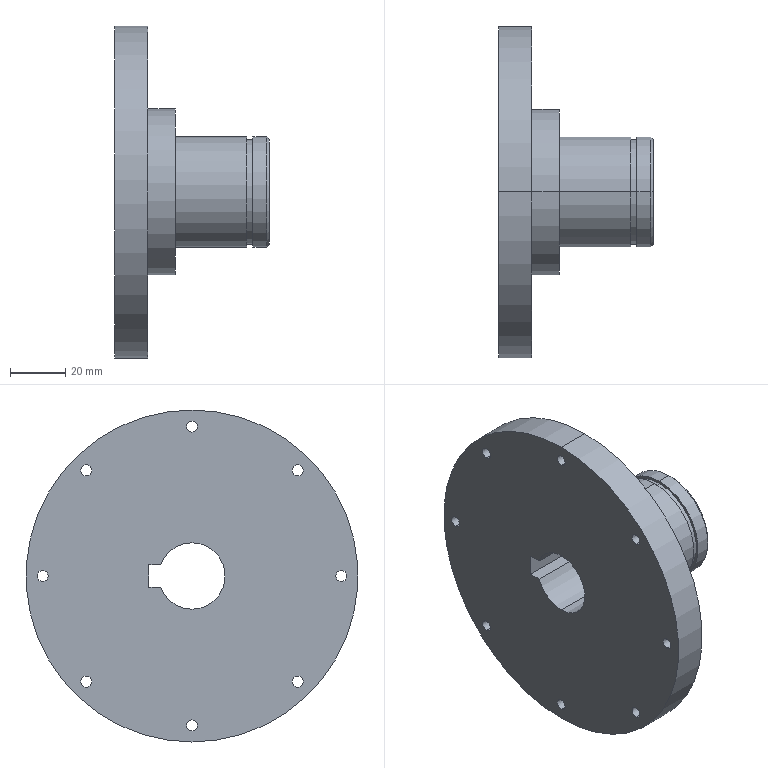Part | SolidWorks | features ICE 3, RevolutionThin 3, Chamfer 1 | 1 solid | 40 faces | box 56 x 120 x 120 mm | volume 178131 mm3 | cylinder 29 | plane 9 | cone 2 | commonest cylinder face diameters 4 x16 40 x4 24 x3 38 x2 60 x2 120 x2
STEP:
#1=CARTESIAN_POINT('',(56.,0.,-19.));
#2=VERTEX_POINT('',#1);
#3=CARTESIAN_POINT('',(56.,0.,19.));
#4=VERTEX_POINT('',#3);
#5=CARTESIAN_POINT('',(56.,0.,0.));
#6=DIRECTION('',(1.,0.,0.));
#7=DIRECTION('',(0.,0.,1.));
#8=AXIS2_PLACEMENT_3D('',#5,#6,#7);
#9=CIRCLE('',#8,19.);
#10=EDGE_CURVE('',#2,#4,#9,.T.);
#11=ORIENTED_EDGE('',*,*,#10,.F.);
#12=CARTESIAN_POINT('',(55.,0.,-20.));
#13=VERTEX_POINT('',#12);
#14=CARTESIAN_POINT('',(55.,0.,-20.));
#15=DIRECTION('',(-0.7071,0.,-0.7071));
#16=VECTOR('',#15,1000.);
#17=LINE('',#14,#16);
#18=EDGE_CURVE('',#2,#13,#17,.T.);
#19=ORIENTED_EDGE('',*,*,#18,.T.);
#20=CARTESIAN_POINT('',(55.,0.,20.));
#21=VERTEX_POINT('',#20);
#22=CARTESIAN_POINT('',(55.,0.,0.));
#23=DIRECTION('',(-1.,0.,0.));
#24=DIRECTION('',(0.,0.,1.));
#25=AXIS2_PLACEMENT_3D('',#22,#23,#24);
#26=CIRCLE('',#25,20.);
#27=EDGE_CURVE('',#21,#13,#26,.T.);
#28=ORIENTED_EDGE('',*,*,#27,.F.);
#29=CARTESIAN_POINT('',(55.,0.,20.));
#30=DIRECTION('',(-0.7071,0.,0.7071));
#31=VECTOR('',#30,1000.);
#32=LINE('',#29,#31);
#33=EDGE_CURVE('',#4,#21,#32,.T.);
#34=ORIENTED_EDGE('',*,*,#33,.F.);
#35=EDGE_LOOP('',(#11,#19,#28,#34));
#36=FACE_OUTER_BOUND('',#35,.T.);
#37=CARTESIAN_POINT('',(55.,0.,0.));
#38=DIRECTION('',(-1.,0.,0.));
#39=DIRECTION('',(0.,0.,1.));
#40=AXIS2_PLACEMENT_3D('',#37,#38,#39);
#41=CONICAL_SURFACE('',#40,20.,0.7854);
#42=ADVANCED_FACE('',(#36),#41,.T.);
#43=CARTESIAN_POINT('',(12.,54.,-2.));
#44=VERTEX_POINT('',#43);
#45=CARTESIAN_POINT('',(12.,54.,2.));
#46=VERTEX_POINT('',#45);
#47=CARTESIAN_POINT('',(12.,54.,0.));
#48=DIRECTION('',(-1.,0.,0.));
#49=DIRECTION('',(0.,0.,1.));
#50=AXIS2_PLACEMENT_3D('',#47,#48,#49);
#51=CIRCLE('',#50,2.);
#52=EDGE_CURVE('',#44,#46,#51,.T.);
#53=ORIENTED_EDGE('',*,*,#52,.F.);
#54=CARTESIAN_POINT('',(0.,54.,-2.));
#55=VERTEX_POINT('',#54);
#56=CARTESIAN_POINT('',(56.,54.,-2.));
#57=DIRECTION('',(-1.,0.,0.));
#58=VECTOR('',#57,1000.);
#59=LINE('',#56,#58);
#60=EDGE_CURVE('',#44,#55,#59,.T.);
#61=ORIENTED_EDGE('',*,*,#60,.T.);
#62=CARTESIAN_POINT('',(0.,54.,2.));
#63=VERTEX_POINT('',#62);
#64=CARTESIAN_POINT('',(0.,54.,0.));
#65=DIRECTION('',(-1.,0.,0.));
#66=DIRECTION('',(0.,0.,1.));
#67=AXIS2_PLACEMENT_3D('',#64,#65,#66);
#68=CIRCLE('',#67,2.);
#69=EDGE_CURVE('',#55,#63,#68,.T.);
#70=ORIENTED_EDGE('',*,*,#69,.T.);
#71=CARTESIAN_POINT('',(56.,54.,2.));
#72=DIRECTION('',(-1.,0.,0.));
#73=VECTOR('',#72,1000.);
#74=LINE('',#71,#73);
#75=EDGE_CURVE('',#46,#63,#74,.T.);
#76=ORIENTED_EDGE('',*,*,#75,.F.);
#77=EDGE_LOOP('',(#53,#61,#70,#76));
#78=FACE_OUTER_BOUND('',#77,.T.);
#79=CARTESIAN_POINT('',(56.,54.,0.));
#80=DIRECTION('',(-1.,0.,0.));
#81=DIRECTION('',(0.,0.,1.));
#82=AXIS2_PLACEMENT_3D('',#79,#80,#81);
#83=CYLINDRICAL_SURFACE('',#82,2.);
#84=ADVANCED_FACE('',(#78),#83,.F.);
#85=CARTESIAN_POINT('',(12.,38.184,36.184));
#86=VERTEX_POINT('',#85);
#87=CARTESIAN_POINT('',(12.,38.184,40.184));
#88=VERTEX_POINT('',#87);
#89=CARTESIAN_POINT('',(12.,38.184,38.184));
#90=DIRECTION('',(-1.,0.,0.));
#91=DIRECTION('',(0.,0.,1.));
#92=AXIS2_PLACEMENT_3D('',#89,#90,#91);
#93=CIRCLE('',#92,2.);
#94=EDGE_CURVE('',#86,#88,#93,.T.);
#95=ORIENTED_EDGE('',*,*,#94,.F.);
#96=CARTESIAN_POINT('',(0.,38.184,36.184));
#97=VERTEX_POINT('',#96);
#98=CARTESIAN_POINT('',(56.,38.184,36.184));
#99=DIRECTION('',(-1.,0.,0.));
#100=VECTOR('',#99,1000.);
#101=LINE('',#98,#100);
#102=EDGE_CURVE('',#86,#97,#101,.T.);
#103=ORIENTED_EDGE('',*,*,#102,.T.);
#104=CARTESIAN_POINT('',(0.,38.184,40.184));
#105=VERTEX_POINT('',#104);
#106=CARTESIAN_POINT('',(0.,38.184,38.184));
#107=DIRECTION('',(-1.,0.,0.));
#108=DIRECTION('',(0.,0.,1.));
#109=AXIS2_PLACEMENT_3D('',#106,#107,#108);
#110=CIRCLE('',#109,2.);
#111=EDGE_CURVE('',#97,#105,#110,.T.);
#112=ORIENTED_EDGE('',*,*,#111,.T.);
#113=CARTESIAN_POINT('',(56.,38.184,40.184));
#114=DIRECTION('',(-1.,0.,0.));
#115=VECTOR('',#114,1000.);
#116=LINE('',#113,#115);
#117=EDGE_CURVE('',#88,#105,#116,.T.);
#118=ORIENTED_EDGE('',*,*,#117,.F.);
#119=EDGE_LOOP('',(#95,#103,#112,#118));
#120=FACE_OUTER_BOUND('',#119,.T.);
#121=CARTESIAN_POINT('',(56.,38.184,38.184));
#122=DIRECTION('',(-1.,0.,0.));
#123=DIRECTION('',(0.,0.,1.));
#124=AXIS2_PLACEMENT_3D('',#121,#122,#123);
#125=CYLINDRICAL_SURFACE('',#124,2.);
#126=ADVANCED_FACE('',(#120),#125,.F.);
#127=CARTESIAN_POINT('',(12.,0.,52.));
#128=VERTEX_POINT('',#127);
#129=CARTESIAN_POINT('',(12.,0.,56.));
#130=VERTEX_POINT('',#129);
#131=CARTESIAN_POINT('',(12.,0.,54.));
#132=DIRECTION('',(-1.,0.,0.));
#133=DIRECTION('',(0.,0.,1.));
#134=AXIS2_PLACEMENT_3D('',#131,#132,#133);
#135=CIRCLE('',#134,2.);
#136=EDGE_CURVE('',#128,#130,#135,.T.);
#137=ORIENTED_EDGE('',*,*,#136,.F.);
#138=CARTESIAN_POINT('',(0.,0.,52.));
#139=VERTEX_POINT('',#138);
#140=CARTESIAN_POINT('',(56.,0.,52.));
#141=DIRECTION('',(-1.,0.,0.));
#142=VECTOR('',#141,1000.);
#143=LINE('',#140,#142);
#144=EDGE_CURVE('',#128,#139,#143,.T.);
#145=ORIENTED_EDGE('',*,*,#144,.T.);
#146=CARTESIAN_POINT('',(0.,0.,56.));
#147=VERTEX_POINT('',#146);
#148=CARTESIAN_POINT('',(0.,0.,54.));
#149=DIRECTION('',(-1.,0.,0.));
#150=DIRECTION('',(0.,0.,1.));
#151=AXIS2_PLACEMENT_3D('',#148,#149,#150);
#152=CIRCLE('',#151,2.);
#153=EDGE_CURVE('',#139,#147,#152,.T.);
#154=ORIENTED_EDGE('',*,*,#153,.T.);
#155=CARTESIAN_POINT('',(56.,0.,56.));
#156=DIRECTION('',(-1.,0.,0.));
#157=VECTOR('',#156,1000.);
#158=LINE('',#155,#157);
#159=EDGE_CURVE('',#130,#147,#158,.T.);
#160=ORIENTED_EDGE('',*,*,#159,.F.);
#161=EDGE_LOOP('',(#137,#145,#154,#160));
#162=FACE_OUTER_BOUND('',#161,.T.);
#163=CARTESIAN_POINT('',(56.,0.,54.));
#164=DIRECTION('',(-1.,0.,0.));
#165=DIRECTION('',(0.,0.,1.));
#166=AXIS2_PLACEMENT_3D('',#163,#164,#165);
#167=CYLINDRICAL_SURFACE('',#166,2.);
#168=ADVANCED_FACE('',(#162),#167,.F.);
#169=CARTESIAN_POINT('',(12.,-38.184,36.184));
#170=VERTEX_POINT('',#169);
#171=CARTESIAN_POINT('',(12.,-38.184,40.184));
#172=VERTEX_POINT('',#171);
#173=CARTESIAN_POINT('',(12.,-38.184,38.184));
#174=DIRECTION('',(-1.,0.,0.));
#175=DIRECTION('',(0.,0.,1.));
#176=AXIS2_PLACEMENT_3D('',#173,#174,#175);
#177=CIRCLE('',#176,2.);
#178=EDGE_CURVE('',#170,#172,#177,.T.);
#179=ORIENTED_EDGE('',*,*,#178,.F.);
#180=CARTESIAN_POINT('',(0.,-38.184,36.184));
#181=VERTEX_POINT('',#180);
#182=CARTESIAN_POINT('',(56.,-38.184,36.184));
#183=DIRECTION('',(-1.,0.,0.));
#184=VECTOR('',#183,1000.);
#185=LINE('',#182,#184);
#186=EDGE_CURVE('',#170,#181,#185,.T.);
#187=ORIENTED_EDGE('',*,*,#186,.T.);
#188=CARTESIAN_POINT('',(0.,-38.184,40.184));
#189=VERTEX_POINT('',#188);
#190=CARTESIAN_POINT('',(0.,-38.184,38.184));
#191=DIRECTION('',(-1.,0.,0.));
#192=DIRECTION('',(0.,0.,1.));
#193=AXIS2_PLACEMENT_3D('',#190,#191,#192);
#194=CIRCLE('',#193,2.);
#195=EDGE_CURVE('',#181,#189,#194,.T.);
#196=ORIENTED_EDGE('',*,*,#195,.T.);
#197=CARTESIAN_POINT('',(56.,-38.184,40.184));
#198=DIRECTION('',(-1.,0.,0.));
#199=VECTOR('',#198,1000.);
#200=LINE('',#197,#199);
#201=EDGE_CURVE('',#172,#189,#200,.T.);
#202=ORIENTED_EDGE('',*,*,#201,.F.);
#203=EDGE_LOOP('',(#179,#187,#196,#202));
#204=FACE_OUTER_BOUND('',#203,.T.);
#205=CARTESIAN_POINT('',(56.,-38.184,38.184));
#206=DIRECTION('',(-1.,0.,0.));
#207=DIRECTION('',(0.,0.,1.));
#208=AXIS2_PLACEMENT_3D('',#205,#206,#207);
#209=CYLINDRICAL_SURFACE('',#208,2.);
#210=ADVANCED_FACE('',(#204),#209,.F.);
#211=CARTESIAN_POINT('',(12.,-54.,-2.));
#212=VERTEX_POINT('',#211);
#213=CARTESIAN_POINT('',(12.,-54.,2.));
#214=VERTEX_POINT('',#213);
#215=CARTESIAN_POINT('',(12.,-54.,0.));
#216=DIRECTION('',(-1.,0.,0.));
#217=DIRECTION('',(0.,0.,1.));
#218=AXIS2_PLACEMENT_3D('',#215,#216,#217);
#219=CIRCLE('',#218,2.);
#220=EDGE_CURVE('',#212,#214,#219,.T.);
#221=ORIENTED_EDGE('',*,*,#220,.F.);
#222=CARTESIAN_POINT('',(0.,-54.,-2.));
#223=VERTEX_POINT('',#222);
#224=CARTESIAN_POINT('',(56.,-54.,-2.));
#225=DIRECTION('',(-1.,0.,0.));
#226=VECTOR('',#225,1000.);
#227=LINE('',#224,#226);
#228=EDGE_CURVE('',#212,#223,#227,.T.);
#229=ORIENTED_EDGE('',*,*,#228,.T.);
#230=CARTESIAN_POINT('',(0.,-54.,2.));
#231=VERTEX_POINT('',#230);
#232=CARTESIAN_POINT('',(0.,-54.,0.));
#233=DIRECTION('',(-1.,0.,0.));
#234=DIRECTION('',(0.,0.,1.));
#235=AXIS2_PLACEMENT_3D('',#232,#233,#234);
#236=CIRCLE('',#235,2.);
#237=EDGE_CURVE('',#223,#231,#236,.T.);
#238=ORIENTED_EDGE('',*,*,#237,.T.);
#239=CARTESIAN_POINT('',(56.,-54.,2.));
#240=DIRECTION('',(-1.,0.,0.));
#241=VECTOR('',#240,1000.);
#242=LINE('',#239,#241);
#243=EDGE_CURVE('',#214,#231,#242,.T.);
#244=ORIENTED_EDGE('',*,*,#243,.F.);
#245=EDGE_LOOP('',(#221,#229,#238,#244));
#246=FACE_OUTER_BOUND('',#245,.T.);
#247=CARTESIAN_POINT('',(56.,-54.,0.));
#248=DIRECTION('',(-1.,0.,0.));
#249=DIRECTION('',(0.,0.,1.));
#250=AXIS2_PLACEMENT_3D('',#247,#248,#249);
#251=CYLINDRICAL_SURFACE('',#250,2.);
#252=ADVANCED_FACE('',(#246),#251,.F.);
#253=CARTESIAN_POINT('',(12.,-38.184,-40.184));
#254=VERTEX_POINT('',#253);
#255=CARTESIAN_POINT('',(12.,-38.184,-36.184));
#256=VERTEX_POINT('',#255);
#257=CARTESIAN_POINT('',(12.,-38.184,-38.184));
#258=DIRECTION('',(-1.,0.,0.));
#259=DIRECTION('',(0.,0.,1.));
#260=AXIS2_PLACEMENT_3D('',#257,#258,#259);
#261=CIRCLE('',#260,2.);
#262=EDGE_CURVE('',#254,#256,#261,.T.);
#263=ORIENTED_EDGE('',*,*,#262,.F.);
#264=CARTESIAN_POINT('',(0.,-38.184,-40.184));
#265=VERTEX_POINT('',#264);
#266=CARTESIAN_POINT('',(56.,-38.184,-40.184));
#267=DIRECTION('',(-1.,0.,0.));
#268=VECTOR('',#267,1000.);
#269=LINE('',#266,#268);
#270=EDGE_CURVE('',#254,#265,#269,.T.);
#271=ORIENTED_EDGE('',*,*,#270,.T.);
#272=CARTESIAN_POINT('',(0.,-38.184,-36.184));
#273=VERTEX_POINT('',#272);
#274=CARTESIAN_POINT('',(0.,-38.184,-38.184));
#275=DIRECTION('',(-1.,0.,0.));
#276=DIRECTION('',(0.,0.,1.));
#277=AXIS2_PLACEMENT_3D('',#274,#275,#276);
#278=CIRCLE('',#277,2.);
#279=EDGE_CURVE('',#265,#273,#278,.T.);
#280=ORIENTED_EDGE('',*,*,#279,.T.);
#281=CARTESIAN_POINT('',(56.,-38.184,-36.184));
#282=DIRECTION('',(-1.,0.,0.));
#283=VECTOR('',#282,1000.);
#284=LINE('',#281,#283);
#285=EDGE_CURVE('',#256,#273,#284,.T.);
#286=ORIENTED_EDGE('',*,*,#285,.F.);
#287=EDGE_LOOP('',(#263,#271,#280,#286));
#288=FACE_OUTER_BOUND('',#287,.T.);
#289=CARTESIAN_POINT('',(56.,-38.184,-38.184));
#290=DIRECTION('',(-1.,0.,0.));
#291=DIRECTION('',(0.,0.,1.));
#292=AXIS2_PLACEMENT_3D('',#289,#290,#291);
#293=CYLINDRICAL_SURFACE('',#292,2.);
#294=ADVANCED_FACE('',(#288),#293,.F.);
#295=CARTESIAN_POINT('',(12.,0.,-56.));
#296=VERTEX_POINT('',#295);
#297=CARTESIAN_POINT('',(12.,0.,-52.));
#298=VERTEX_POINT('',#297);
#299=CARTESIAN_POINT('',(12.,0.,-54.));
#300=DIRECTION('',(-1.,0.,0.));
#301=DIRECTION('',(0.,0.,1.));
#302=AXIS2_PLACEMENT_3D('',#299,#300,#301);
#303=CIRCLE('',#302,2.);
#304=EDGE_CURVE('',#296,#298,#303,.T.);
#305=ORIENTED_EDGE('',*,*,#304,.F.);
#306=CARTESIAN_POINT('',(0.,0.,-56.));
#307=VERTEX_POINT('',#306);
#308=CARTESIAN_POINT('',(56.,0.,-56.));
#309=DIRECTION('',(-1.,0.,0.));
#310=VECTOR('',#309,1000.);
#311=LINE('',#308,#310);
#312=EDGE_CURVE('',#296,#307,#311,.T.);
#313=ORIENTED_EDGE('',*,*,#312,.T.);
#314=CARTESIAN_POINT('',(0.,0.,-52.));
#315=VERTEX_POINT('',#314);
#316=CARTESIAN_POINT('',(0.,0.,-54.));
#317=DIRECTION('',(-1.,0.,0.));
#318=DIRECTION('',(0.,0.,1.));
#319=AXIS2_PLACEMENT_3D('',#316,#317,#318);
#320=CIRCLE('',#319,2.);
#321=EDGE_CURVE('',#307,#315,#320,.T.);
#322=ORIENTED_EDGE('',*,*,#321,.T.);
#323=CARTESIAN_POINT('',(56.,0.,-52.));
#324=DIRECTION('',(-1.,0.,0.));
#325=VECTOR('',#324,1000.);
#326=LINE('',#323,#325);
#327=EDGE_CURVE('',#298,#315,#326,.T.);
#328=ORIENTED_EDGE('',*,*,#327,.F.);
#329=EDGE_LOOP('',(#305,#313,#322,#328));
#330=FACE_OUTER_BOUND('',#329,.T.);
#331=CARTESIAN_POINT('',(56.,0.,-54.));
#332=DIRECTION('',(-1.,0.,0.));
#333=DIRECTION('',(0.,0.,1.));
#334=AXIS2_PLACEMENT_3D('',#331,#332,#333);
#335=CYLINDRICAL_SURFACE('',#334,2.);
#336=ADVANCED_FACE('',(#330),#335,.F.);
#337=CARTESIAN_POINT('',(12.,38.184,-40.184));
#338=VERTEX_POINT('',#337);
#339=CARTESIAN_POINT('',(12.,38.184,-36.184));
#340=VERTEX_POINT('',#339);
#341=CARTESIAN_POINT('',(12.,38.184,-38.184));
#342=DIRECTION('',(-1.,0.,0.));
#343=DIRECTION('',(0.,0.,1.));
#344=AXIS2_PLACEMENT_3D('',#341,#342,#343);
#345=CIRCLE('',#344,2.);
#346=EDGE_CURVE('',#338,#340,#345,.T.);
#347=ORIENTED_EDGE('',*,*,#346,.F.);
#348=CARTESIAN_POINT('',(0.,38.184,-40.184));
#349=VERTEX_POINT('',#348);
#350=CARTESIAN_POINT('',(56.,38.184,-40.184));
#351=DIRECTION('',(-1.,0.,0.));
#352=VECTOR('',#351,1000.);
#353=LINE('',#350,#352);
#354=EDGE_CURVE('',#338,#349,#353,.T.);
#355=ORIENTED_EDGE('',*,*,#354,.T.);
#356=CARTESIAN_POINT('',(0.,38.184,-36.184));
#357=VERTEX_POINT('',#356);
#358=CARTESIAN_POINT('',(0.,38.184,-38.184));
#359=DIRECTION('',(-1.,0.,0.));
#360=DIRECTION('',(0.,0.,1.));
#361=AXIS2_PLACEMENT_3D('',#358,#359,#360);
#362=CIRCLE('',#361,2.);
#363=EDGE_CURVE('',#349,#357,#362,.T.);
#364=ORIENTED_EDGE('',*,*,#363,.T.);
#365=CARTESIAN_POINT('',(56.,38.184,-36.184));
#366=DIRECTION('',(-1.,0.,0.));
#367=VECTOR('',#366,1000.);
#368=LINE('',#365,#367);
#369=EDGE_CURVE('',#340,#357,#368,.T.);
#370=ORIENTED_EDGE('',*,*,#369,.F.);
#371=EDGE_LOOP('',(#347,#355,#364,#370));
#372=FACE_OUTER_BOUND('',#371,.T.);
#373=CARTESIAN_POINT('',(56.,38.184,-38.184));
#374=DIRECTION('',(-1.,0.,0.));
#375=DIRECTION('',(0.,0.,1.));
#376=AXIS2_PLACEMENT_3D('',#373,#374,#375);
#377=CYLINDRICAL_SURFACE('',#376,2.);
#378=ADVANCED_FACE('',(#372),#377,.F.);
#379=CARTESIAN_POINT('',(47.8,0.,-19.));
#380=VERTEX_POINT('',#379);
#381=CARTESIAN_POINT('',(47.8,0.,19.));
#382=VERTEX_POINT('',#381);
#383=CARTESIAN_POINT('',(47.8,0.,0.));
#384=DIRECTION('',(1.,0.,0.));
#385=DIRECTION('',(0.,0.,-1.));
#386=AXIS2_PLACEMENT_3D('',#383,#384,#385);
#387=CIRCLE('',#386,19.);
#388=EDGE_CURVE('',#380,#382,#387,.T.);
#389=ORIENTED_EDGE('',*,*,#388,.T.);
#390=CARTESIAN_POINT('',(50.,0.,19.));
#391=VERTEX_POINT('',#390);
#392=CARTESIAN_POINT('',(47.8,0.,19.));
#393=DIRECTION('',(1.,0.,0.));
#394=VECTOR('',#393,1000.);
#395=LINE('',#392,#394);
#396=EDGE_CURVE('',#382,#391,#395,.T.);
#397=ORIENTED_EDGE('',*,*,#396,.T.);
#398=CARTESIAN_POINT('',(50.,0.,-19.));
#399=VERTEX_POINT('',#398);
#400=CARTESIAN_POINT('',(50.,0.,0.));
#401=DIRECTION('',(1.,0.,0.));
#402=DIRECTION('',(0.,0.,-1.));
#403=AXIS2_PLACEMENT_3D('',#400,#401,#402);
#404=CIRCLE('',#403,19.);
#405=EDGE_CURVE('',#399,#391,#404,.T.);
#406=ORIENTED_EDGE('',*,*,#405,.F.);
#407=CARTESIAN_POINT('',(47.8,0.,-19.));
#408=DIRECTION('',(1.,0.,0.));
#409=VECTOR('',#408,1000.);
#410=LINE('',#407,#409);
#411=EDGE_CURVE('',#380,#399,#410,.T.);
#412=ORIENTED_EDGE('',*,*,#411,.F.);
#413=EDGE_LOOP('',(#389,#397,#406,#412));
#414=FACE_OUTER_BOUND('',#413,.T.);
#415=CARTESIAN_POINT('',(47.8,0.,0.));
#416=DIRECTION('',(1.,0.,0.));
#417=DIRECTION('',(0.,0.,-1.));
#418=AXIS2_PLACEMENT_3D('',#415,#416,#417);
#419=CYLINDRICAL_SURFACE('',#418,19.);
#420=ADVANCED_FACE('',(#414),#419,.T.);
#421=CARTESIAN_POINT('',(56.,0.,12.));
#422=VERTEX_POINT('',#421);
#423=CARTESIAN_POINT('',(56.,0.,-12.));
#424=VERTEX_POINT('',#423);
#425=CARTESIAN_POINT('',(56.,0.,0.));
#426=DIRECTION('',(1.,0.,0.));
#427=DIRECTION('',(0.,0.,-1.));
#428=AXIS2_PLACEMENT_3D('',#425,#426,#427);
#429=CIRCLE('',#428,12.);
#430=EDGE_CURVE('',#422,#424,#429,.T.);
#431=ORIENTED_EDGE('',*,*,#430,.T.);
#432=CARTESIAN_POINT('',(0.,0.,-12.));
#433=VERTEX_POINT('',#432);
#434=CARTESIAN_POINT('',(56.,0.,-12.));
#435=DIRECTION('',(-1.,0.,0.));
#436=VECTOR('',#435,1000.);
#437=LINE('',#434,#436);
#438=EDGE_CURVE('',#424,#433,#437,.T.);
#439=ORIENTED_EDGE('',*,*,#438,.T.);
#440=CARTESIAN_POINT('',(0.,0.,12.));
#441=VERTEX_POINT('',#440);
#442=CARTESIAN_POINT('',(0.,0.,0.));
#443=DIRECTION('',(1.,0.,0.));
#444=DIRECTION('',(0.,0.,-1.));
#445=AXIS2_PLACEMENT_3D('',#442,#443,#444);
#446=CIRCLE('',#445,12.);
#447=EDGE_CURVE('',#441,#433,#446,.T.);
#448=ORIENTED_EDGE('',*,*,#447,.F.);
#449=CARTESIAN_POINT('',(56.,0.,12.));
#450=DIRECTION('',(-1.,0.,0.));
#451=VECTOR('',#450,1000.);
#452=LINE('',#449,#451);
#453=EDGE_CURVE('',#422,#441,#452,.T.);
#454=ORIENTED_EDGE('',*,*,#453,.F.);
#455=EDGE_LOOP('',(#431,#439,#448,#454));
#456=FACE_OUTER_BOUND('',#455,.T.);
#457=CARTESIAN_POINT('',(56.,0.,0.));
#458=DIRECTION('',(-1.,0.,0.));
#459=DIRECTION('',(0.,0.,1.));
#460=AXIS2_PLACEMENT_3D('',#457,#458,#459);
#461=CYLINDRICAL_SURFACE('',#460,12.);
#462=ADVANCED_FACE('',(#456),#461,.F.);
#463=CARTESIAN_POINT('',(56.,11.314,4.));
#464=VERTEX_POINT('',#463);
#465=CARTESIAN_POINT('',(56.,0.,0.));
#466=DIRECTION('',(1.,0.,0.));
#467=DIRECTION('',(0.,0.,-1.));
#468=AXIS2_PLACEMENT_3D('',#465,#466,#467);
#469=CIRCLE('',#468,12.);
#470=EDGE_CURVE('',#464,#422,#469,.T.);
#471=ORIENTED_EDGE('',*,*,#470,.T.);
#472=ORIENTED_EDGE('',*,*,#453,.T.);
#473=CARTESIAN_POINT('',(0.,11.314,4.));
#474=VERTEX_POINT('',#473);
#475=CARTESIAN_POINT('',(0.,0.,0.));
#476=DIRECTION('',(1.,0.,0.));
#477=DIRECTION('',(0.,0.,-1.));
#478=AXIS2_PLACEMENT_3D('',#475,#476,#477);
#479=CIRCLE('',#478,12.);
#480=EDGE_CURVE('',#474,#441,#479,.T.);
#481=ORIENTED_EDGE('',*,*,#480,.F.);
#482=CARTESIAN_POINT('',(56.,11.314,4.));
#483=DIRECTION('',(-1.,0.,0.));
#484=VECTOR('',#483,1000.);
#485=LINE('',#482,#484);
#486=EDGE_CURVE('',#464,#474,#485,.T.);
#487=ORIENTED_EDGE('',*,*,#486,.F.);
#488=EDGE_LOOP('',(#471,#472,#481,#487));
#489=FACE_OUTER_BOUND('',#488,.T.);
#490=CARTESIAN_POINT('',(56.,0.,0.));
#491=DIRECTION('',(-1.,0.,0.));
#492=DIRECTION('',(0.,0.,1.));
#493=AXIS2_PLACEMENT_3D('',#490,#491,#492);
#494=CYLINDRICAL_SURFACE('',#493,12.);
#495=ADVANCED_FACE('',(#489),#494,.F.);
#496=ORIENTED_EDGE('',*,*,#27,.T.);
#497=CARTESIAN_POINT('',(50.,0.,-20.));
#498=VERTEX_POINT('',#497);
#499=CARTESIAN_POINT('',(22.,0.,-20.));
#500=DIRECTION('',(-1.,0.,0.));
#501=VECTOR('',#500,1000.);
#502=LINE('',#499,#501);
#503=EDGE_CURVE('',#13,#498,#502,.T.);
#504=ORIENTED_EDGE('',*,*,#503,.T.);
#505=CARTESIAN_POINT('',(50.,0.,20.));
#506=VERTEX_POINT('',#505);
#507=CARTESIAN_POINT('',(50.,0.,0.));
#508=DIRECTION('',(-1.,0.,0.));
#509=DIRECTION('',(0.,0.,-1.));
#510=AXIS2_PLACEMENT_3D('',#507,#508,#509);
#511=CIRCLE('',#510,20.);
#512=EDGE_CURVE('',#506,#498,#511,.T.);
#513=ORIENTED_EDGE('',*,*,#512,.F.);
#514=CARTESIAN_POINT('',(22.,0.,20.));
#515=DIRECTION('',(-1.,0.,0.));
#516=VECTOR('',#515,1000.);
#517=LINE('',#514,#516);
#518=EDGE_CURVE('',#21,#506,#517,.T.);
#519=ORIENTED_EDGE('',*,*,#518,.F.);
#520=EDGE_LOOP('',(#496,#504,#513,#519));
#521=FACE_OUTER_BOUND('',#520,.T.);
#522=CARTESIAN_POINT('',(22.,0.,0.));
#523=DIRECTION('',(-1.,0.,0.));
#524=DIRECTION('',(0.,0.,1.));
#525=AXIS2_PLACEMENT_3D('',#522,#523,#524);
#526=CYLINDRICAL_SURFACE('',#525,20.);
#527=ADVANCED_FACE('',(#521),#526,.T.);
#528=CARTESIAN_POINT('',(22.,0.,30.));
#529=VERTEX_POINT('',#528);
#530=CARTESIAN_POINT('',(22.,0.,-30.));
#531=VERTEX_POINT('',#530);
#532=CARTESIAN_POINT('',(22.,0.,0.));
#533=DIRECTION('',(-1.,0.,0.));
#534=DIRECTION('',(0.,0.,1.));
#535=AXIS2_PLACEMENT_3D('',#532,#533,#534);
#536=CIRCLE('',#535,30.);
#537=EDGE_CURVE('',#529,#531,#536,.T.);
#538=ORIENTED_EDGE('',*,*,#537,.T.);
#539=CARTESIAN_POINT('',(12.,0.,-30.));
#540=VERTEX_POINT('',#539);
#541=CARTESIAN_POINT('',(12.,0.,-30.));
#542=DIRECTION('',(-1.,0.,0.));
#543=VECTOR('',#542,1000.);
#544=LINE('',#541,#543);
#545=EDGE_CURVE('',#531,#540,#544,.T.);
#546=ORIENTED_EDGE('',*,*,#545,.T.);
#547=CARTESIAN_POINT('',(12.,0.,30.));
#548=VERTEX_POINT('',#547);
#549=CARTESIAN_POINT('',(12.,0.,0.));
#550=DIRECTION('',(-1.,0.,0.));
#551=DIRECTION('',(0.,0.,1.));
#552=AXIS2_PLACEMENT_3D('',#549,#550,#551);
#553=CIRCLE('',#552,30.);
#554=EDGE_CURVE('',#548,#540,#553,.T.);
#555=ORIENTED_EDGE('',*,*,#554,.F.);
#556=CARTESIAN_POINT('',(12.,0.,30.));
#557=DIRECTION('',(-1.,0.,0.));
#558=VECTOR('',#557,1000.);
#559=LINE('',#556,#558);
#560=EDGE_CURVE('',#529,#548,#559,.T.);
#561=ORIENTED_EDGE('',*,*,#560,.F.);
#562=EDGE_LOOP('',(#538,#546,#555,#561));
#563=FACE_OUTER_BOUND('',#562,.T.);
#564=CARTESIAN_POINT('',(12.,0.,0.));
#565=DIRECTION('',(-1.,0.,0.));
#566=DIRECTION('',(0.,0.,1.));
#567=AXIS2_PLACEMENT_3D('',#564,#565,#566);
#568=CYLINDRICAL_SURFACE('',#567,30.);
#569=ADVANCED_FACE('',(#563),#568,.T.);
#570=CARTESIAN_POINT('',(12.,0.,60.));
#571=VERTEX_POINT('',#570);
#572=CARTESIAN_POINT('',(12.,0.,-60.));
#573=VERTEX_POINT('',#572);
#574=CARTESIAN_POINT('',(12.,0.,0.));
#575=DIRECTION('',(-1.,0.,0.));
#576=DIRECTION('',(0.,0.,1.));
#577=AXIS2_PLACEMENT_3D('',#574,#575,#576);
#578=CIRCLE('',#577,60.);
#579=EDGE_CURVE('',#571,#573,#578,.T.);
#580=ORIENTED_EDGE('',*,*,#579,.T.);
#581=CARTESIAN_POINT('',(0.,0.,-60.));
#582=VERTEX_POINT('',#581);
#583=CARTESIAN_POINT('',(0.,0.,-60.));
#584=DIRECTION('',(-1.,0.,0.));
#585=VECTOR('',#584,1000.);
#586=LINE('',#583,#585);
#587=EDGE_CURVE('',#573,#582,#586,.T.);
#588=ORIENTED_EDGE('',*,*,#587,.T.);
#589=CARTESIAN_POINT('',(0.,0.,60.));
#590=VERTEX_POINT('',#589);
#591=CARTESIAN_POINT('',(0.,0.,0.));
#592=DIRECTION('',(-1.,0.,0.));
#593=DIRECTION('',(0.,0.,1.));
#594=AXIS2_PLACEMENT_3D('',#591,#592,#593);
#595=CIRCLE('',#594,60.);
#596=EDGE_CURVE('',#590,#582,#595,.T.);
#597=ORIENTED_EDGE('',*,*,#596,.F.);
#598=CARTESIAN_POINT('',(0.,0.,60.));
#599=DIRECTION('',(-1.,0.,0.));
#600=VECTOR('',#599,1000.);
#601=LINE('',#598,#600);
#602=EDGE_CURVE('',#571,#590,#601,.T.);
#603=ORIENTED_EDGE('',*,*,#602,.F.);
#604=EDGE_LOOP('',(#580,#588,#597,#603));
#605=FACE_OUTER_BOUND('',#604,.T.);
#606=CARTESIAN_POINT('',(0.,0.,0.));
#607=DIRECTION('',(-1.,0.,0.));
#608=DIRECTION('',(0.,0.,1.));
#609=AXIS2_PLACEMENT_3D('',#606,#607,#608);
#610=CYLINDRICAL_SURFACE('',#609,60.);
#611=ADVANCED_FACE('',(#605),#610,.T.);
#612=CARTESIAN_POINT('',(47.8,0.,20.));
#613=VERTEX_POINT('',#612);
#614=CARTESIAN_POINT('',(47.8,0.,-20.));
#615=VERTEX_POINT('',#614);
#616=CARTESIAN_POINT('',(47.8,0.,0.));
#617=DIRECTION('',(-1.,0.,0.));
#618=DIRECTION('',(0.,0.,-1.));
#619=AXIS2_PLACEMENT_3D('',#616,#617,#618);
#620=CIRCLE('',#619,20.);
#621=EDGE_CURVE('',#613,#615,#620,.T.);
#622=ORIENTED_EDGE('',*,*,#621,.T.);
#623=CARTESIAN_POINT('',(22.,0.,-20.));
#624=VERTEX_POINT('',#623);
#625=CARTESIAN_POINT('',(22.,0.,-20.));
#626=DIRECTION('',(-1.,0.,0.));
#627=VECTOR('',#626,1000.);
#628=LINE('',#625,#627);
#629=EDGE_CURVE('',#615,#624,#628,.T.);
#630=ORIENTED_EDGE('',*,*,#629,.T.);
#631=CARTESIAN_POINT('',(22.,0.,20.));
#632=VERTEX_POINT('',#631);
#633=CARTESIAN_POINT('',(22.,0.,0.));
#634=DIRECTION('',(-1.,0.,0.));
#635=DIRECTION('',(0.,0.,1.));
#636=AXIS2_PLACEMENT_3D('',#633,#634,#635);
#637=CIRCLE('',#636,20.);
#638=EDGE_CURVE('',#632,#624,#637,.T.);
#639=ORIENTED_EDGE('',*,*,#638,.F.);
#640=CARTESIAN_POINT('',(22.,0.,20.));
#641=DIRECTION('',(-1.,0.,0.));
#642=VECTOR('',#641,1000.);
#643=LINE('',#640,#642);
#644=EDGE_CURVE('',#613,#632,#643,.T.);
#645=ORIENTED_EDGE('',*,*,#644,.F.);
#646=EDGE_LOOP('',(#622,#630,#639,#645));
#647=FACE_OUTER_BOUND('',#646,.T.);
#648=CARTESIAN_POINT('',(22.,0.,0.));
#649=DIRECTION('',(-1.,0.,0.));
#650=DIRECTION('',(0.,0.,1.));
#651=AXIS2_PLACEMENT_3D('',#648,#649,#650);
#652=CYLINDRICAL_SURFACE('',#651,20.);
#653=ADVANCED_FACE('',(#647),#652,.T.);
#654=ORIENTED_EDGE('',*,*,#629,.F.);
#655=CARTESIAN_POINT('',(47.8,0.,0.));
#656=DIRECTION('',(-1.,0.,0.));
#657=DIRECTION('',(0.,0.,-1.));
#658=AXIS2_PLACEMENT_3D('',#655,#656,#657);
#659=CIRCLE('',#658,20.);
#660=EDGE_CURVE('',#615,#613,#659,.T.);
#661=ORIENTED_EDGE('',*,*,#660,.T.);
#662=ORIENTED_EDGE('',*,*,#644,.T.);
#663=CARTESIAN_POINT('',(22.,0.,0.));
#664=DIRECTION('',(-1.,0.,0.));
#665=DIRECTION('',(0.,0.,1.));
#666=AXIS2_PLACEMENT_3D('',#663,#664,#665);
#667=CIRCLE('',#666,20.);
#668=EDGE_CURVE('',#624,#632,#667,.T.);
#669=ORIENTED_EDGE('',*,*,#668,.F.);
#670=EDGE_LOOP('',(#654,#661,#662,#669));
#671=FACE_OUTER_BOUND('',#670,.T.);
#672=CARTESIAN_POINT('',(22.,0.,0.));
#673=DIRECTION('',(-1.,0.,0.));
#674=DIRECTION('',(0.,0.,1.));
#675=AXIS2_PLACEMENT_3D('',#672,#673,#674);
#676=CYLINDRICAL_SURFACE('',#675,20.);
#677=ADVANCED_FACE('',(#671),#676,.T.);
#678=ORIENTED_EDGE('',*,*,#587,.F.);
#679=CARTESIAN_POINT('',(12.,0.,0.));
#680=DIRECTION('',(-1.,0.,0.));
#681=DIRECTION('',(0.,0.,1.));
#682=AXIS2_PLACEMENT_3D('',#679,#680,#681);
#683=CIRCLE('',#682,60.);
#684=EDGE_CURVE('',#573,#571,#683,.T.);
#685=ORIENTED_EDGE('',*,*,#684,.T.);
#686=ORIENTED_EDGE('',*,*,#602,.T.);
#687=CARTESIAN_POINT('',(0.,0.,0.));
#688=DIRECTION('',(-1.,0.,0.));
#689=DIRECTION('',(0.,0.,1.));
#690=AXIS2_PLACEMENT_3D('',#687,#688,#689);
#691=CIRCLE('',#690,60.);
#692=EDGE_CURVE('',#582,#590,#691,.T.);
#693=ORIENTED_EDGE('',*,*,#692,.F.);
#694=EDGE_LOOP('',(#678,#685,#686,#693));
#695=FACE_OUTER_BOUND('',#694,.T.);
#696=CARTESIAN_POINT('',(0.,0.,0.));
#697=DIRECTION('',(-1.,0.,0.));
#698=DIRECTION('',(0.,0.,1.));
#699=AXIS2_PLACEMENT_3D('',#696,#697,#698);
#700=CYLINDRICAL_SURFACE('',#699,60.);
#701=ADVANCED_FACE('',(#695),#700,.T.);
#702=CARTESIAN_POINT('',(0.,54.,0.));
#703=DIRECTION('',(-1.,0.,0.));
#704=DIRECTION('',(0.,0.,1.));
#705=AXIS2_PLACEMENT_3D('',#702,#703,#704);
#706=CIRCLE('',#705,2.);
#707=EDGE_CURVE('',#63,#55,#706,.T.);
#708=ORIENTED_EDGE('',*,*,#707,.F.);
#709=ORIENTED_EDGE('',*,*,#69,.F.);
#710=EDGE_LOOP('',(#708,#709));
#711=FACE_BOUND('',#710,.T.);
#712=CARTESIAN_POINT('',(0.,38.184,38.184));
#713=DIRECTION('',(-1.,0.,0.));
#714=DIRECTION('',(0.,0.,1.));
#715=AXIS2_PLACEMENT_3D('',#712,#713,#714);
#716=CIRCLE('',#715,2.);
#717=EDGE_CURVE('',#105,#97,#716,.T.);
#718=ORIENTED_EDGE('',*,*,#717,.F.);
#719=ORIENTED_EDGE('',*,*,#111,.F.);
#720=EDGE_LOOP('',(#718,#719));
#721=FACE_BOUND('',#720,.T.);
#722=CARTESIAN_POINT('',(0.,0.,54.));
#723=DIRECTION('',(-1.,0.,0.));
#724=DIRECTION('',(0.,0.,1.));
#725=AXIS2_PLACEMENT_3D('',#722,#723,#724);
#726=CIRCLE('',#725,2.);
#727=EDGE_CURVE('',#147,#139,#726,.T.);
#728=ORIENTED_EDGE('',*,*,#727,.F.);
#729=ORIENTED_EDGE('',*,*,#153,.F.);
#730=EDGE_LOOP('',(#728,#729));
#731=FACE_BOUND('',#730,.T.);
#732=CARTESIAN_POINT('',(0.,-38.184,38.184));
#733=DIRECTION('',(-1.,0.,0.));
#734=DIRECTION('',(0.,0.,1.));
#735=AXIS2_PLACEMENT_3D('',#732,#733,#734);
#736=CIRCLE('',#735,2.);
#737=EDGE_CURVE('',#189,#181,#736,.T.);
#738=ORIENTED_EDGE('',*,*,#737,.F.);
#739=ORIENTED_EDGE('',*,*,#195,.F.);
#740=EDGE_LOOP('',(#738,#739));
#741=FACE_BOUND('',#740,.T.);
#742=CARTESIAN_POINT('',(0.,-54.,0.));
#743=DIRECTION('',(-1.,0.,0.));
#744=DIRECTION('',(0.,0.,1.));
#745=AXIS2_PLACEMENT_3D('',#742,#743,#744);
#746=CIRCLE('',#745,2.);
#747=EDGE_CURVE('',#231,#223,#746,.T.);
#748=ORIENTED_EDGE('',*,*,#747,.F.);
#749=ORIENTED_EDGE('',*,*,#237,.F.);
#750=EDGE_LOOP('',(#748,#749));
#751=FACE_BOUND('',#750,.T.);
#752=CARTESIAN_POINT('',(0.,-38.184,-38.184));
#753=DIRECTION('',(-1.,0.,0.));
#754=DIRECTION('',(0.,0.,1.));
#755=AXIS2_PLACEMENT_3D('',#752,#753,#754);
#756=CIRCLE('',#755,2.);
#757=EDGE_CURVE('',#273,#265,#756,.T.);
#758=ORIENTED_EDGE('',*,*,#757,.F.);
#759=ORIENTED_EDGE('',*,*,#279,.F.);
#760=EDGE_LOOP('',(#758,#759));
#761=FACE_BOUND('',#760,.T.);
#762=CARTESIAN_POINT('',(0.,0.,-54.));
#763=DIRECTION('',(-1.,0.,0.));
#764=DIRECTION('',(0.,0.,1.));
#765=AXIS2_PLACEMENT_3D('',#762,#763,#764);
#766=CIRCLE('',#765,2.);
#767=EDGE_CURVE('',#315,#307,#766,.T.);
#768=ORIENTED_EDGE('',*,*,#767,.F.);
#769=ORIENTED_EDGE('',*,*,#321,.F.);
#770=EDGE_LOOP('',(#768,#769));
#771=FACE_BOUND('',#770,.T.);
#772=CARTESIAN_POINT('',(0.,38.184,-38.184));
#773=DIRECTION('',(-1.,0.,0.));
#774=DIRECTION('',(0.,0.,1.));
#775=AXIS2_PLACEMENT_3D('',#772,#773,#774);
#776=CIRCLE('',#775,2.);
#777=EDGE_CURVE('',#357,#349,#776,.T.);
#778=ORIENTED_EDGE('',*,*,#777,.F.);
#779=ORIENTED_EDGE('',*,*,#363,.F.);
#780=EDGE_LOOP('',(#778,#779));
#781=FACE_BOUND('',#780,.T.);
#782=CARTESIAN_POINT('',(0.,11.314,-4.));
#783=VERTEX_POINT('',#782);
#784=CARTESIAN_POINT('',(0.,15.6,-4.));
#785=VERTEX_POINT('',#784);
#786=CARTESIAN_POINT('',(0.,15.6,-4.));
#787=DIRECTION('',(0.,1.,0.));
#788=VECTOR('',#787,1000.);
#789=LINE('',#786,#788);
#790=EDGE_CURVE('',#783,#785,#789,.T.);
#791=ORIENTED_EDGE('',*,*,#790,.T.);
#792=CARTESIAN_POINT('',(0.,15.6,4.));
#793=VERTEX_POINT('',#792);
#794=CARTESIAN_POINT('',(0.,15.6,4.));
#795=DIRECTION('',(0.,0.,1.));
#796=VECTOR('',#795,1000.);
#797=LINE('',#794,#796);
#798=EDGE_CURVE('',#785,#793,#797,.T.);
#799=ORIENTED_EDGE('',*,*,#798,.T.);
#800=CARTESIAN_POINT('',(0.,15.6,4.));
#801=DIRECTION('',(0.,-1.,0.));
#802=VECTOR('',#801,1000.);
#803=LINE('',#800,#802);
#804=EDGE_CURVE('',#793,#474,#803,.T.);
#805=ORIENTED_EDGE('',*,*,#804,.T.);
#806=ORIENTED_EDGE('',*,*,#480,.T.);
#807=ORIENTED_EDGE('',*,*,#447,.T.);
#808=CARTESIAN_POINT('',(0.,0.,0.));
#809=DIRECTION('',(1.,0.,0.));
#810=DIRECTION('',(0.,0.,-1.));
#811=AXIS2_PLACEMENT_3D('',#808,#809,#810);
#812=CIRCLE('',#811,12.);
#813=EDGE_CURVE('',#433,#783,#812,.T.);
#814=ORIENTED_EDGE('',*,*,#813,.T.);
#815=EDGE_LOOP('',(#791,#799,#805,#806,#807,#814));
#816=FACE_BOUND('',#815,.T.);
#817=ORIENTED_EDGE('',*,*,#596,.T.);
#818=ORIENTED_EDGE('',*,*,#692,.T.);
#819=EDGE_LOOP('',(#817,#818));
#820=FACE_OUTER_BOUND('',#819,.T.);
#821=CARTESIAN_POINT('',(0.,-60.,0.));
#822=DIRECTION('',(1.,0.,0.));
#823=DIRECTION('',(0.,0.,-1.));
#824=AXIS2_PLACEMENT_3D('',#821,#822,#823);
#825=PLANE('',#824);
#826=ADVANCED_FACE('',(#711,#721,#731,#741,#751,#761,#771,#781,#816,#820),#825,.F.);
#827=CARTESIAN_POINT('',(12.,54.,0.));
#828=DIRECTION('',(-1.,0.,0.));
#829=DIRECTION('',(0.,0.,1.));
#830=AXIS2_PLACEMENT_3D('',#827,#828,#829);
#831=CIRCLE('',#830,2.);
#832=EDGE_CURVE('',#46,#44,#831,.T.);
#833=ORIENTED_EDGE('',*,*,#832,.T.);
#834=ORIENTED_EDGE('',*,*,#52,.T.);
#835=EDGE_LOOP('',(#833,#834));
#836=FACE_BOUND('',#835,.T.);
#837=CARTESIAN_POINT('',(12.,38.184,38.184));
#838=DIRECTION('',(-1.,0.,0.));
#839=DIRECTION('',(0.,0.,1.));
#840=AXIS2_PLACEMENT_3D('',#837,#838,#839);
#841=CIRCLE('',#840,2.);
#842=EDGE_CURVE('',#88,#86,#841,.T.);
#843=ORIENTED_EDGE('',*,*,#842,.T.);
#844=ORIENTED_EDGE('',*,*,#94,.T.);
#845=EDGE_LOOP('',(#843,#844));
#846=FACE_BOUND('',#845,.T.);
#847=CARTESIAN_POINT('',(12.,0.,54.));
#848=DIRECTION('',(-1.,0.,0.));
#849=DIRECTION('',(0.,0.,1.));
#850=AXIS2_PLACEMENT_3D('',#847,#848,#849);
#851=CIRCLE('',#850,2.);
#852=EDGE_CURVE('',#130,#128,#851,.T.);
#853=ORIENTED_EDGE('',*,*,#852,.T.);
#854=ORIENTED_EDGE('',*,*,#136,.T.);
#855=EDGE_LOOP('',(#853,#854));
#856=FACE_BOUND('',#855,.T.);
#857=CARTESIAN_POINT('',(12.,-38.184,38.184));
#858=DIRECTION('',(-1.,0.,0.));
#859=DIRECTION('',(0.,0.,1.));
#860=AXIS2_PLACEMENT_3D('',#857,#858,#859);
#861=CIRCLE('',#860,2.);
#862=EDGE_CURVE('',#172,#170,#861,.T.);
#863=ORIENTED_EDGE('',*,*,#862,.T.);
#864=ORIENTED_EDGE('',*,*,#178,.T.);
#865=EDGE_LOOP('',(#863,#864));
#866=FACE_BOUND('',#865,.T.);
#867=CARTESIAN_POINT('',(12.,-54.,0.));
#868=DIRECTION('',(-1.,0.,0.));
#869=DIRECTION('',(0.,0.,1.));
#870=AXIS2_PLACEMENT_3D('',#867,#868,#869);
#871=CIRCLE('',#870,2.);
#872=EDGE_CURVE('',#214,#212,#871,.T.);
#873=ORIENTED_EDGE('',*,*,#872,.T.);
#874=ORIENTED_EDGE('',*,*,#220,.T.);
#875=EDGE_LOOP('',(#873,#874));
#876=FACE_BOUND('',#875,.T.);
#877=CARTESIAN_POINT('',(12.,-38.184,-38.184));
#878=DIRECTION('',(-1.,0.,0.));
#879=DIRECTION('',(0.,0.,1.));
#880=AXIS2_PLACEMENT_3D('',#877,#878,#879);
#881=CIRCLE('',#880,2.);
#882=EDGE_CURVE('',#256,#254,#881,.T.);
#883=ORIENTED_EDGE('',*,*,#882,.T.);
#884=ORIENTED_EDGE('',*,*,#262,.T.);
#885=EDGE_LOOP('',(#883,#884));
#886=FACE_BOUND('',#885,.T.);
#887=CARTESIAN_POINT('',(12.,0.,-54.));
#888=DIRECTION('',(-1.,0.,0.));
#889=DIRECTION('',(0.,0.,1.));
#890=AXIS2_PLACEMENT_3D('',#887,#888,#889);
#891=CIRCLE('',#890,2.);
#892=EDGE_CURVE('',#298,#296,#891,.T.);
#893=ORIENTED_EDGE('',*,*,#892,.T.);
#894=ORIENTED_EDGE('',*,*,#304,.T.);
#895=EDGE_LOOP('',(#893,#894));
#896=FACE_BOUND('',#895,.T.);
#897=CARTESIAN_POINT('',(12.,38.184,-38.184));
#898=DIRECTION('',(-1.,0.,0.));
#899=DIRECTION('',(0.,0.,1.));
#900=AXIS2_PLACEMENT_3D('',#897,#898,#899);
#901=CIRCLE('',#900,2.);
#902=EDGE_CURVE('',#340,#338,#901,.T.);
#903=ORIENTED_EDGE('',*,*,#902,.T.);
#904=ORIENTED_EDGE('',*,*,#346,.T.);
#905=EDGE_LOOP('',(#903,#904));
#906=FACE_BOUND('',#905,.T.);
#907=ORIENTED_EDGE('',*,*,#554,.T.);
#908=CARTESIAN_POINT('',(12.,0.,0.));
#909=DIRECTION('',(-1.,0.,0.));
#910=DIRECTION('',(0.,0.,1.));
#911=AXIS2_PLACEMENT_3D('',#908,#909,#910);
#912=CIRCLE('',#911,30.);
#913=EDGE_CURVE('',#540,#548,#912,.T.);
#914=ORIENTED_EDGE('',*,*,#913,.T.);
#915=EDGE_LOOP('',(#907,#914));
#916=FACE_BOUND('',#915,.T.);
#917=ORIENTED_EDGE('',*,*,#579,.F.);
#918=ORIENTED_EDGE('',*,*,#684,.F.);
#919=EDGE_LOOP('',(#917,#918));
#920=FACE_OUTER_BOUND('',#919,.T.);
#921=CARTESIAN_POINT('',(12.,0.,0.));
#922=DIRECTION('',(-1.,0.,0.));
#923=DIRECTION('',(0.,0.,1.));
#924=AXIS2_PLACEMENT_3D('',#921,#922,#923);
#925=PLANE('',#924);
#926=ADVANCED_FACE('',(#836,#846,#856,#866,#876,#886,#896,#906,#916,#920),#925,.F.);
#927=ORIENTED_EDGE('',*,*,#545,.F.);
#928=CARTESIAN_POINT('',(22.,0.,0.));
#929=DIRECTION('',(-1.,0.,0.));
#930=DIRECTION('',(0.,0.,1.));
#931=AXIS2_PLACEMENT_3D('',#928,#929,#930);
#932=CIRCLE('',#931,30.);
#933=EDGE_CURVE('',#531,#529,#932,.T.);
#934=ORIENTED_EDGE('',*,*,#933,.T.);
#935=ORIENTED_EDGE('',*,*,#560,.T.);
#936=ORIENTED_EDGE('',*,*,#913,.F.);
#937=EDGE_LOOP('',(#927,#934,#935,#936));
#938=FACE_OUTER_BOUND('',#937,.T.);
#939=CARTESIAN_POINT('',(12.,0.,0.));
#940=DIRECTION('',(-1.,0.,0.));
#941=DIRECTION('',(0.,0.,1.));
#942=AXIS2_PLACEMENT_3D('',#939,#940,#941);
#943=CYLINDRICAL_SURFACE('',#942,30.);
#944=ADVANCED_FACE('',(#938),#943,.T.);
#945=ORIENTED_EDGE('',*,*,#638,.T.);
#946=ORIENTED_EDGE('',*,*,#668,.T.);
#947=EDGE_LOOP('',(#945,#946));
#948=FACE_BOUND('',#947,.T.);
#949=ORIENTED_EDGE('',*,*,#537,.F.);
#950=ORIENTED_EDGE('',*,*,#933,.F.);
#951=EDGE_LOOP('',(#949,#950));
#952=FACE_OUTER_BOUND('',#951,.T.);
#953=CARTESIAN_POINT('',(22.,0.,0.));
#954=DIRECTION('',(-1.,0.,0.));
#955=DIRECTION('',(0.,0.,1.));
#956=AXIS2_PLACEMENT_3D('',#953,#954,#955);
#957=PLANE('',#956);
#958=ADVANCED_FACE('',(#948,#952),#957,.F.);
#959=ORIENTED_EDGE('',*,*,#503,.F.);
#960=CARTESIAN_POINT('',(55.,0.,0.));
#961=DIRECTION('',(-1.,0.,0.));
#962=DIRECTION('',(0.,0.,1.));
#963=AXIS2_PLACEMENT_3D('',#960,#961,#962);
#964=CIRCLE('',#963,20.);
#965=EDGE_CURVE('',#13,#21,#964,.T.);
#966=ORIENTED_EDGE('',*,*,#965,.T.);
#967=ORIENTED_EDGE('',*,*,#518,.T.);
#968=CARTESIAN_POINT('',(50.,0.,0.));
#969=DIRECTION('',(-1.,0.,0.));
#970=DIRECTION('',(0.,0.,-1.));
#971=AXIS2_PLACEMENT_3D('',#968,#969,#970);
#972=CIRCLE('',#971,20.);
#973=EDGE_CURVE('',#498,#506,#972,.T.);
#974=ORIENTED_EDGE('',*,*,#973,.F.);
#975=EDGE_LOOP('',(#959,#966,#967,#974));
#976=FACE_OUTER_BOUND('',#975,.T.);
#977=CARTESIAN_POINT('',(22.,0.,0.));
#978=DIRECTION('',(-1.,0.,0.));
#979=DIRECTION('',(0.,0.,1.));
#980=AXIS2_PLACEMENT_3D('',#977,#978,#979);
#981=CYLINDRICAL_SURFACE('',#980,20.);
#982=ADVANCED_FACE('',(#976),#981,.T.);
#983=CARTESIAN_POINT('',(56.,0.,0.));
#984=DIRECTION('',(1.,0.,0.));
#985=DIRECTION('',(0.,0.,1.));
#986=AXIS2_PLACEMENT_3D('',#983,#984,#985);
#987=CIRCLE('',#986,19.);
#988=EDGE_CURVE('',#4,#2,#987,.T.);
#989=ORIENTED_EDGE('',*,*,#988,.T.);
#990=ORIENTED_EDGE('',*,*,#10,.T.);
#991=EDGE_LOOP('',(#989,#990));
#992=FACE_OUTER_BOUND('',#991,.T.);
#993=CARTESIAN_POINT('',(56.,11.314,-4.));
#994=VERTEX_POINT('',#993);
#995=CARTESIAN_POINT('',(56.,15.6,-4.));
#996=VERTEX_POINT('',#995);
#997=CARTESIAN_POINT('',(56.,15.6,-4.));
#998=DIRECTION('',(0.,1.,0.));
#999=VECTOR('',#998,1000.);
#1000=LINE('',#997,#999);
#1001=EDGE_CURVE('',#994,#996,#1000,.T.);
#1002=ORIENTED_EDGE('',*,*,#1001,.F.);
#1003=CARTESIAN_POINT('',(56.,0.,0.));
#1004=DIRECTION('',(1.,0.,0.));
#1005=DIRECTION('',(0.,0.,-1.));
#1006=AXIS2_PLACEMENT_3D('',#1003,#1004,#1005);
#1007=CIRCLE('',#1006,12.);
#1008=EDGE_CURVE('',#424,#994,#1007,.T.);
#1009=ORIENTED_EDGE('',*,*,#1008,.F.);
#1010=ORIENTED_EDGE('',*,*,#430,.F.);
#1011=ORIENTED_EDGE('',*,*,#470,.F.);
#1012=CARTESIAN_POINT('',(56.,15.6,4.));
#1013=VERTEX_POINT('',#1012);
#1014=CARTESIAN_POINT('',(56.,15.6,4.));
#1015=DIRECTION('',(0.,-1.,0.));
#1016=VECTOR('',#1015,1000.);
#1017=LINE('',#1014,#1016);
#1018=EDGE_CURVE('',#1013,#464,#1017,.T.);
#1019=ORIENTED_EDGE('',*,*,#1018,.F.);
#1020=CARTESIAN_POINT('',(56.,15.6,4.));
#1021=DIRECTION('',(0.,0.,1.));
#1022=VECTOR('',#1021,1000.);
#1023=LINE('',#1020,#1022);
#1024=EDGE_CURVE('',#996,#1013,#1023,.T.);
#1025=ORIENTED_EDGE('',*,*,#1024,.F.);
#1026=EDGE_LOOP('',(#1002,#1009,#1010,#1011,#1019,#1025));
#1027=FACE_BOUND('',#1026,.T.);
#1028=CARTESIAN_POINT('',(56.,0.,0.));
#1029=DIRECTION('',(-1.,0.,0.));
#1030=DIRECTION('',(0.,0.,1.));
#1031=AXIS2_PLACEMENT_3D('',#1028,#1029,#1030);
#1032=PLANE('',#1031);
#1033=ADVANCED_FACE('',(#992,#1027),#1032,.F.);
#1034=ORIENTED_EDGE('',*,*,#790,.F.);
#1035=CARTESIAN_POINT('',(56.,11.314,-4.));
#1036=DIRECTION('',(-1.,0.,0.));
#1037=VECTOR('',#1036,1000.);
#1038=LINE('',#1035,#1037);
#1039=EDGE_CURVE('',#994,#783,#1038,.T.);
#1040=ORIENTED_EDGE('',*,*,#1039,.F.);
#1041=ORIENTED_EDGE('',*,*,#1001,.T.);
#1042=CARTESIAN_POINT('',(56.,15.6,-4.));
#1043=DIRECTION('',(-1.,0.,0.));
#1044=VECTOR('',#1043,1000.);
#1045=LINE('',#1042,#1044);
#1046=EDGE_CURVE('',#996,#785,#1045,.T.);
#1047=ORIENTED_EDGE('',*,*,#1046,.T.);
#1048=EDGE_LOOP('',(#1034,#1040,#1041,#1047));
#1049=FACE_OUTER_BOUND('',#1048,.T.);
#1050=CARTESIAN_POINT('',(56.,15.6,-4.));
#1051=DIRECTION('',(0.,0.,1.));
#1052=DIRECTION('',(1.,0.,0.));
#1053=AXIS2_PLACEMENT_3D('',#1050,#1051,#1052);
#1054=PLANE('',#1053);
#1055=ADVANCED_FACE('',(#1049),#1054,.T.);
#1056=ORIENTED_EDGE('',*,*,#798,.F.);
#1057=ORIENTED_EDGE('',*,*,#1046,.F.);
#1058=ORIENTED_EDGE('',*,*,#1024,.T.);
#1059=CARTESIAN_POINT('',(56.,15.6,4.));
#1060=DIRECTION('',(-1.,0.,0.));
#1061=VECTOR('',#1060,1000.);
#1062=LINE('',#1059,#1061);
#1063=EDGE_CURVE('',#1013,#793,#1062,.T.);
#1064=ORIENTED_EDGE('',*,*,#1063,.T.);
#1065=EDGE_LOOP('',(#1056,#1057,#1058,#1064));
#1066=FACE_OUTER_BOUND('',#1065,.T.);
#1067=CARTESIAN_POINT('',(56.,15.6,4.));
#1068=DIRECTION('',(0.,-1.,0.));
#1069=DIRECTION('',(0.,0.,-1.));
#1070=AXIS2_PLACEMENT_3D('',#1067,#1068,#1069);
#1071=PLANE('',#1070);
#1072=ADVANCED_FACE('',(#1066),#1071,.T.);
#1073=ORIENTED_EDGE('',*,*,#804,.F.);
#1074=ORIENTED_EDGE('',*,*,#1063,.F.);
#1075=ORIENTED_EDGE('',*,*,#1018,.T.);
#1076=ORIENTED_EDGE('',*,*,#486,.T.);
#1077=EDGE_LOOP('',(#1073,#1074,#1075,#1076));
#1078=FACE_OUTER_BOUND('',#1077,.T.);
#1079=CARTESIAN_POINT('',(56.,15.6,4.));
#1080=DIRECTION('',(0.,0.,-1.));
#1081=DIRECTION('',(-1.,0.,0.));
#1082=AXIS2_PLACEMENT_3D('',#1079,#1080,#1081);
#1083=PLANE('',#1082);
#1084=ADVANCED_FACE('',(#1078),#1083,.T.);
#1085=ORIENTED_EDGE('',*,*,#438,.F.);
#1086=ORIENTED_EDGE('',*,*,#1008,.T.);
#1087=ORIENTED_EDGE('',*,*,#1039,.T.);
#1088=ORIENTED_EDGE('',*,*,#813,.F.);
#1089=EDGE_LOOP('',(#1085,#1086,#1087,#1088));
#1090=FACE_OUTER_BOUND('',#1089,.T.);
#1091=CARTESIAN_POINT('',(56.,0.,0.));
#1092=DIRECTION('',(-1.,0.,0.));
#1093=DIRECTION('',(0.,0.,1.));
#1094=AXIS2_PLACEMENT_3D('',#1091,#1092,#1093);
#1095=CYLINDRICAL_SURFACE('',#1094,12.);
#1096=ADVANCED_FACE('',(#1090),#1095,.F.);
#1097=ORIENTED_EDGE('',*,*,#621,.F.);
#1098=ORIENTED_EDGE('',*,*,#660,.F.);
#1099=EDGE_LOOP('',(#1097,#1098));
#1100=FACE_OUTER_BOUND('',#1099,.T.);
#1101=ORIENTED_EDGE('',*,*,#388,.F.);
#1102=CARTESIAN_POINT('',(47.8,0.,0.));
#1103=DIRECTION('',(1.,0.,0.));
#1104=DIRECTION('',(0.,0.,-1.));
#1105=AXIS2_PLACEMENT_3D('',#1102,#1103,#1104);
#1106=CIRCLE('',#1105,19.);
#1107=EDGE_CURVE('',#382,#380,#1106,.T.);
#1108=ORIENTED_EDGE('',*,*,#1107,.F.);
#1109=EDGE_LOOP('',(#1101,#1108));
#1110=FACE_BOUND('',#1109,.T.);
#1111=CARTESIAN_POINT('',(47.8,0.,0.));
#1112=DIRECTION('',(1.,0.,0.));
#1113=DIRECTION('',(0.,0.,-1.));
#1114=AXIS2_PLACEMENT_3D('',#1111,#1112,#1113);
#1115=PLANE('',#1114);
#1116=ADVANCED_FACE('',(#1100,#1110),#1115,.T.);
#1117=ORIENTED_EDGE('',*,*,#512,.T.);
#1118=ORIENTED_EDGE('',*,*,#973,.T.);
#1119=EDGE_LOOP('',(#1117,#1118));
#1120=FACE_OUTER_BOUND('',#1119,.T.);
#1121=ORIENTED_EDGE('',*,*,#405,.T.);
#1122=CARTESIAN_POINT('',(50.,0.,0.));
#1123=DIRECTION('',(1.,0.,0.));
#1124=DIRECTION('',(0.,0.,-1.));
#1125=AXIS2_PLACEMENT_3D('',#1122,#1123,#1124);
#1126=CIRCLE('',#1125,19.);
#1127=EDGE_CURVE('',#391,#399,#1126,.T.);
#1128=ORIENTED_EDGE('',*,*,#1127,.T.);
#1129=EDGE_LOOP('',(#1121,#1128));
#1130=FACE_BOUND('',#1129,.T.);
#1131=CARTESIAN_POINT('',(50.,0.,0.));
#1132=DIRECTION('',(1.,0.,0.));
#1133=DIRECTION('',(0.,0.,-1.));
#1134=AXIS2_PLACEMENT_3D('',#1131,#1132,#1133);
#1135=PLANE('',#1134);
#1136=ADVANCED_FACE('',(#1120,#1130),#1135,.F.);
#1137=ORIENTED_EDGE('',*,*,#396,.F.);
#1138=ORIENTED_EDGE('',*,*,#1107,.T.);
#1139=ORIENTED_EDGE('',*,*,#411,.T.);
#1140=ORIENTED_EDGE('',*,*,#1127,.F.);
#1141=EDGE_LOOP('',(#1137,#1138,#1139,#1140));
#1142=FACE_OUTER_BOUND('',#1141,.T.);
#1143=CARTESIAN_POINT('',(47.8,0.,0.));
#1144=DIRECTION('',(1.,0.,0.));
#1145=DIRECTION('',(0.,0.,-1.));
#1146=AXIS2_PLACEMENT_3D('',#1143,#1144,#1145);
#1147=CYLINDRICAL_SURFACE('',#1146,19.);
#1148=ADVANCED_FACE('',(#1142),#1147,.T.);
#1149=ORIENTED_EDGE('',*,*,#354,.F.);
#1150=ORIENTED_EDGE('',*,*,#902,.F.);
#1151=ORIENTED_EDGE('',*,*,#369,.T.);
#1152=ORIENTED_EDGE('',*,*,#777,.T.);
#1153=EDGE_LOOP('',(#1149,#1150,#1151,#1152));
#1154=FACE_OUTER_BOUND('',#1153,.T.);
#1155=CARTESIAN_POINT('',(56.,38.184,-38.184));
#1156=DIRECTION('',(-1.,0.,0.));
#1157=DIRECTION('',(0.,0.,1.));
#1158=AXIS2_PLACEMENT_3D('',#1155,#1156,#1157);
#1159=CYLINDRICAL_SURFACE('',#1158,2.);
#1160=ADVANCED_FACE('',(#1154),#1159,.F.);
#1161=ORIENTED_EDGE('',*,*,#312,.F.);
#1162=ORIENTED_EDGE('',*,*,#892,.F.);
#1163=ORIENTED_EDGE('',*,*,#327,.T.);
#1164=ORIENTED_EDGE('',*,*,#767,.T.);
#1165=EDGE_LOOP('',(#1161,#1162,#1163,#1164));
#1166=FACE_OUTER_BOUND('',#1165,.T.);
#1167=CARTESIAN_POINT('',(56.,0.,-54.));
#1168=DIRECTION('',(-1.,0.,0.));
#1169=DIRECTION('',(0.,0.,1.));
#1170=AXIS2_PLACEMENT_3D('',#1167,#1168,#1169);
#1171=CYLINDRICAL_SURFACE('',#1170,2.);
#1172=ADVANCED_FACE('',(#1166),#1171,.F.);
#1173=ORIENTED_EDGE('',*,*,#270,.F.);
#1174=ORIENTED_EDGE('',*,*,#882,.F.);
#1175=ORIENTED_EDGE('',*,*,#285,.T.);
#1176=ORIENTED_EDGE('',*,*,#757,.T.);
#1177=EDGE_LOOP('',(#1173,#1174,#1175,#1176));
#1178=FACE_OUTER_BOUND('',#1177,.T.);
#1179=CARTESIAN_POINT('',(56.,-38.184,-38.184));
#1180=DIRECTION('',(-1.,0.,0.));
#1181=DIRECTION('',(0.,0.,1.));
#1182=AXIS2_PLACEMENT_3D('',#1179,#1180,#1181);
#1183=CYLINDRICAL_SURFACE('',#1182,2.);
#1184=ADVANCED_FACE('',(#1178),#1183,.F.);
#1185=ORIENTED_EDGE('',*,*,#228,.F.);
#1186=ORIENTED_EDGE('',*,*,#872,.F.);
#1187=ORIENTED_EDGE('',*,*,#243,.T.);
#1188=ORIENTED_EDGE('',*,*,#747,.T.);
#1189=EDGE_LOOP('',(#1185,#1186,#1187,#1188));
#1190=FACE_OUTER_BOUND('',#1189,.T.);
#1191=CARTESIAN_POINT('',(56.,-54.,0.));
#1192=DIRECTION('',(-1.,0.,0.));
#1193=DIRECTION('',(0.,0.,1.));
#1194=AXIS2_PLACEMENT_3D('',#1191,#1192,#1193);
#1195=CYLINDRICAL_SURFACE('',#1194,2.);
#1196=ADVANCED_FACE('',(#1190),#1195,.F.);
#1197=ORIENTED_EDGE('',*,*,#186,.F.);
#1198=ORIENTED_EDGE('',*,*,#862,.F.);
#1199=ORIENTED_EDGE('',*,*,#201,.T.);
#1200=ORIENTED_EDGE('',*,*,#737,.T.);
#1201=EDGE_LOOP('',(#1197,#1198,#1199,#1200));
#1202=FACE_OUTER_BOUND('',#1201,.T.);
#1203=CARTESIAN_POINT('',(56.,-38.184,38.184));
#1204=DIRECTION('',(-1.,0.,0.));
#1205=DIRECTION('',(0.,0.,1.));
#1206=AXIS2_PLACEMENT_3D('',#1203,#1204,#1205);
#1207=CYLINDRICAL_SURFACE('',#1206,2.);
#1208=ADVANCED_FACE('',(#1202),#1207,.F.);
#1209=ORIENTED_EDGE('',*,*,#144,.F.);
#1210=ORIENTED_EDGE('',*,*,#852,.F.);
#1211=ORIENTED_EDGE('',*,*,#159,.T.);
#1212=ORIENTED_EDGE('',*,*,#727,.T.);
#1213=EDGE_LOOP('',(#1209,#1210,#1211,#1212));
#1214=FACE_OUTER_BOUND('',#1213,.T.);
#1215=CARTESIAN_POINT('',(56.,0.,54.));
#1216=DIRECTION('',(-1.,0.,0.));
#1217=DIRECTION('',(0.,0.,1.));
#1218=AXIS2_PLACEMENT_3D('',#1215,#1216,#1217);
#1219=CYLINDRICAL_SURFACE('',#1218,2.);
#1220=ADVANCED_FACE('',(#1214),#1219,.F.);
#1221=ORIENTED_EDGE('',*,*,#102,.F.);
#1222=ORIENTED_EDGE('',*,*,#842,.F.);
#1223=ORIENTED_EDGE('',*,*,#117,.T.);
#1224=ORIENTED_EDGE('',*,*,#717,.T.);
#1225=EDGE_LOOP('',(#1221,#1222,#1223,#1224));
#1226=FACE_OUTER_BOUND('',#1225,.T.);
#1227=CARTESIAN_POINT('',(56.,38.184,38.184));
#1228=DIRECTION('',(-1.,0.,0.));
#1229=DIRECTION('',(0.,0.,1.));
#1230=AXIS2_PLACEMENT_3D('',#1227,#1228,#1229);
#1231=CYLINDRICAL_SURFACE('',#1230,2.);
#1232=ADVANCED_FACE('',(#1226),#1231,.F.);
#1233=ORIENTED_EDGE('',*,*,#60,.F.);
#1234=ORIENTED_EDGE('',*,*,#832,.F.);
#1235=ORIENTED_EDGE('',*,*,#75,.T.);
#1236=ORIENTED_EDGE('',*,*,#707,.T.);
#1237=EDGE_LOOP('',(#1233,#1234,#1235,#1236));
#1238=FACE_OUTER_BOUND('',#1237,.T.);
#1239=CARTESIAN_POINT('',(56.,54.,0.));
#1240=DIRECTION('',(-1.,0.,0.));
#1241=DIRECTION('',(0.,0.,1.));
#1242=AXIS2_PLACEMENT_3D('',#1239,#1240,#1241);
#1243=CYLINDRICAL_SURFACE('',#1242,2.);
#1244=ADVANCED_FACE('',(#1238),#1243,.F.);
#1245=ORIENTED_EDGE('',*,*,#18,.F.);
#1246=ORIENTED_EDGE('',*,*,#988,.F.);
#1247=ORIENTED_EDGE('',*,*,#33,.T.);
#1248=ORIENTED_EDGE('',*,*,#965,.F.);
#1249=EDGE_LOOP('',(#1245,#1246,#1247,#1248));
#1250=FACE_OUTER_BOUND('',#1249,.T.);
#1251=CARTESIAN_POINT('',(55.,0.,0.));
#1252=DIRECTION('',(-1.,0.,0.));
#1253=DIRECTION('',(0.,0.,1.));
#1254=AXIS2_PLACEMENT_3D('',#1251,#1252,#1253);
#1255=CONICAL_SURFACE('',#1254,20.,0.7854);
#1256=ADVANCED_FACE('',(#1250),#1255,.T.);
#1257=CLOSED_SHELL('',(#42,#84,#126,#168,#210,#252,#294,#336,#378,#420,#462,#495,#527,#569,#611,#653,#677,#701,#826,#926,#944,#958,#982,#1033,#1055,#1072,#1084,#1096,#1116,#1136,#1148,#1160,#1172,#1184,#1196,#1208,#1220,#1232,#1244,#1256));
#1258=MANIFOLD_SOLID_BREP('',#1257);
#1259=CARTESIAN_POINT('',(0.,0.,0.));
#1260=DIRECTION('',(0.,0.,1.));
#1261=DIRECTION('',(1.,0.,0.));
#1262=AXIS2_PLACEMENT_3D('',#1259,#1260,#1261);
#1263=(LENGTH_UNIT()NAMED_UNIT(*)SI_UNIT(.MILLI.,.METRE.));
#1264=UNCERTAINTY_MEASURE_WITH_UNIT(LENGTH_MEASURE(0.00001),#1263,'','');
#1265=(NAMED_UNIT(*)PLANE_ANGLE_UNIT()SI_UNIT($,.RADIAN.));
#1266=(NAMED_UNIT(*)SI_UNIT($,.STERADIAN.)SOLID_ANGLE_UNIT());
#1267=(GEOMETRIC_REPRESENTATION_CONTEXT(3)GLOBAL_UNCERTAINTY_ASSIGNED_CONTEXT((#1264))GLOBAL_UNIT_ASSIGNED_CONTEXT((#1263,#1265,#1266))REPRESENTATION_CONTEXT('',''));
#1268=ADVANCED_BREP_SHAPE_REPRESENTATION('',(#1258,#1262),#1267);